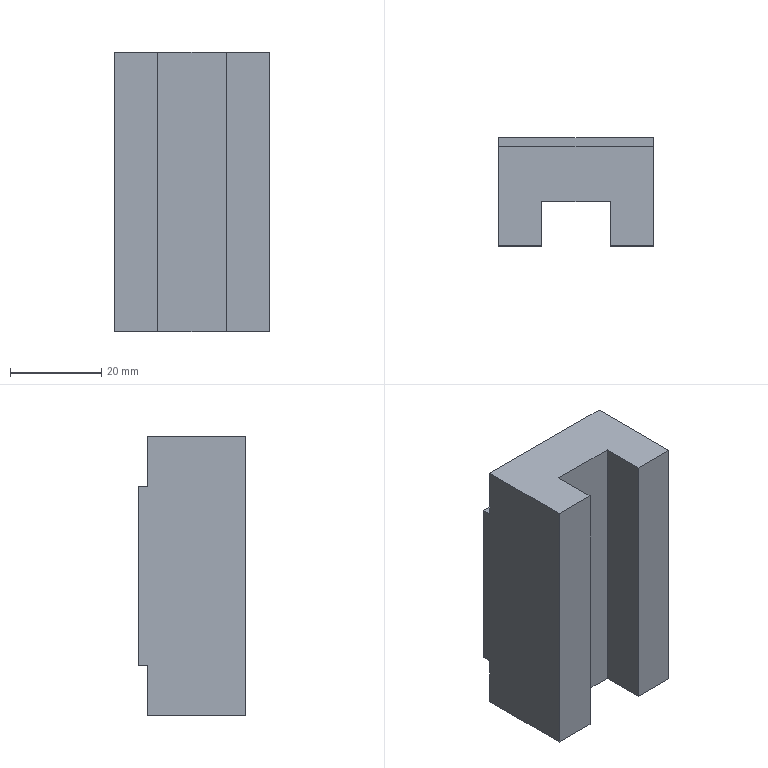Part | STEP file | PN_0044 (HGH15CA block) | 1 solid | 30 faces | box 34 x 23.7 x 61.4 mm | volume 38690 mm3 | plane 14 | cylinder 8 | cone 8 | commonest cylinder face diameters 3.3 x8